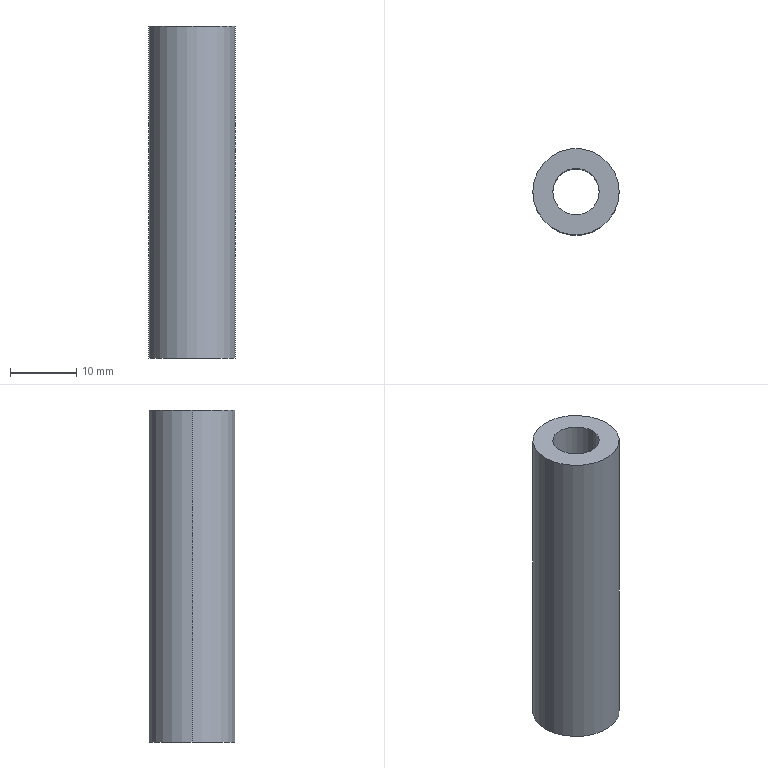Part | SolidWorks | features Extrusion 1 | 1 solid | 6 faces | box 13 x 13 x 50 mm | volume 4712 mm3 | cylinder 4 | plane 2 | commonest cylinder face diameters 7 x2 13 x2
STEP:
#1=CARTESIAN_POINT('',(-3.5,0.,50.));
#2=VERTEX_POINT('',#1);
#3=CARTESIAN_POINT('',(3.5,0.,50.));
#4=VERTEX_POINT('',#3);
#5=CARTESIAN_POINT('',(0.,0.,50.));
#6=DIRECTION('',(0.,0.,1.));
#7=DIRECTION('',(1.,0.,0.));
#8=AXIS2_PLACEMENT_3D('',#5,#6,#7);
#9=CIRCLE('',#8,3.5);
#10=EDGE_CURVE('',#2,#4,#9,.T.);
#11=ORIENTED_EDGE('',*,*,#10,.T.);
#12=CARTESIAN_POINT('',(3.5,0.,0.));
#13=VERTEX_POINT('',#12);
#14=CARTESIAN_POINT('',(3.5,0.,50.));
#15=DIRECTION('',(0.,0.,-1.));
#16=VECTOR('',#15,1000.);
#17=LINE('',#14,#16);
#18=EDGE_CURVE('',#4,#13,#17,.T.);
#19=ORIENTED_EDGE('',*,*,#18,.T.);
#20=CARTESIAN_POINT('',(-3.5,0.,0.));
#21=VERTEX_POINT('',#20);
#22=CARTESIAN_POINT('',(0.,0.,0.));
#23=DIRECTION('',(0.,0.,1.));
#24=DIRECTION('',(1.,0.,0.));
#25=AXIS2_PLACEMENT_3D('',#22,#23,#24);
#26=CIRCLE('',#25,3.5);
#27=EDGE_CURVE('',#21,#13,#26,.T.);
#28=ORIENTED_EDGE('',*,*,#27,.F.);
#29=CARTESIAN_POINT('',(-3.5,0.,50.));
#30=DIRECTION('',(0.,0.,-1.));
#31=VECTOR('',#30,1000.);
#32=LINE('',#29,#31);
#33=EDGE_CURVE('',#2,#21,#32,.T.);
#34=ORIENTED_EDGE('',*,*,#33,.F.);
#35=EDGE_LOOP('',(#11,#19,#28,#34));
#36=FACE_OUTER_BOUND('',#35,.T.);
#37=CARTESIAN_POINT('',(0.,0.,50.));
#38=DIRECTION('',(0.,0.,-1.));
#39=DIRECTION('',(-1.,0.,0.));
#40=AXIS2_PLACEMENT_3D('',#37,#38,#39);
#41=CYLINDRICAL_SURFACE('',#40,3.5);
#42=ADVANCED_FACE('',(#36),#41,.F.);
#43=CARTESIAN_POINT('',(6.5,0.,50.));
#44=VERTEX_POINT('',#43);
#45=CARTESIAN_POINT('',(-6.5,0.,50.));
#46=VERTEX_POINT('',#45);
#47=CARTESIAN_POINT('',(0.,0.,50.));
#48=DIRECTION('',(0.,0.,1.));
#49=DIRECTION('',(1.,0.,0.));
#50=AXIS2_PLACEMENT_3D('',#47,#48,#49);
#51=CIRCLE('',#50,6.5);
#52=EDGE_CURVE('',#44,#46,#51,.T.);
#53=ORIENTED_EDGE('',*,*,#52,.F.);
#54=CARTESIAN_POINT('',(6.5,0.,0.));
#55=VERTEX_POINT('',#54);
#56=CARTESIAN_POINT('',(6.5,0.,50.));
#57=DIRECTION('',(0.,0.,-1.));
#58=VECTOR('',#57,1000.);
#59=LINE('',#56,#58);
#60=EDGE_CURVE('',#44,#55,#59,.T.);
#61=ORIENTED_EDGE('',*,*,#60,.T.);
#62=CARTESIAN_POINT('',(-6.5,0.,0.));
#63=VERTEX_POINT('',#62);
#64=CARTESIAN_POINT('',(0.,0.,0.));
#65=DIRECTION('',(0.,0.,1.));
#66=DIRECTION('',(1.,0.,0.));
#67=AXIS2_PLACEMENT_3D('',#64,#65,#66);
#68=CIRCLE('',#67,6.5);
#69=EDGE_CURVE('',#55,#63,#68,.T.);
#70=ORIENTED_EDGE('',*,*,#69,.T.);
#71=CARTESIAN_POINT('',(-6.5,0.,50.));
#72=DIRECTION('',(0.,0.,-1.));
#73=VECTOR('',#72,1000.);
#74=LINE('',#71,#73);
#75=EDGE_CURVE('',#46,#63,#74,.T.);
#76=ORIENTED_EDGE('',*,*,#75,.F.);
#77=EDGE_LOOP('',(#53,#61,#70,#76));
#78=FACE_OUTER_BOUND('',#77,.T.);
#79=CARTESIAN_POINT('',(0.,0.,50.));
#80=DIRECTION('',(0.,0.,-1.));
#81=DIRECTION('',(-1.,0.,0.));
#82=AXIS2_PLACEMENT_3D('',#79,#80,#81);
#83=CYLINDRICAL_SURFACE('',#82,6.5);
#84=ADVANCED_FACE('',(#78),#83,.T.);
#85=CARTESIAN_POINT('',(0.,0.,50.));
#86=DIRECTION('',(0.,0.,1.));
#87=DIRECTION('',(1.,0.,0.));
#88=AXIS2_PLACEMENT_3D('',#85,#86,#87);
#89=CIRCLE('',#88,6.5);
#90=EDGE_CURVE('',#46,#44,#89,.T.);
#91=ORIENTED_EDGE('',*,*,#90,.T.);
#92=ORIENTED_EDGE('',*,*,#52,.T.);
#93=EDGE_LOOP('',(#91,#92));
#94=FACE_OUTER_BOUND('',#93,.T.);
#95=ORIENTED_EDGE('',*,*,#10,.F.);
#96=CARTESIAN_POINT('',(0.,0.,50.));
#97=DIRECTION('',(0.,0.,1.));
#98=DIRECTION('',(1.,0.,0.));
#99=AXIS2_PLACEMENT_3D('',#96,#97,#98);
#100=CIRCLE('',#99,3.5);
#101=EDGE_CURVE('',#4,#2,#100,.T.);
#102=ORIENTED_EDGE('',*,*,#101,.F.);
#103=EDGE_LOOP('',(#95,#102));
#104=FACE_BOUND('',#103,.T.);
#105=CARTESIAN_POINT('',(0.,0.,50.));
#106=DIRECTION('',(0.,0.,1.));
#107=DIRECTION('',(1.,0.,0.));
#108=AXIS2_PLACEMENT_3D('',#105,#106,#107);
#109=PLANE('',#108);
#110=ADVANCED_FACE('',(#94,#104),#109,.T.);
#111=CARTESIAN_POINT('',(0.,0.,0.));
#112=DIRECTION('',(0.,0.,1.));
#113=DIRECTION('',(1.,0.,0.));
#114=AXIS2_PLACEMENT_3D('',#111,#112,#113);
#115=CIRCLE('',#114,6.5);
#116=EDGE_CURVE('',#63,#55,#115,.T.);
#117=ORIENTED_EDGE('',*,*,#116,.F.);
#118=ORIENTED_EDGE('',*,*,#69,.F.);
#119=EDGE_LOOP('',(#117,#118));
#120=FACE_OUTER_BOUND('',#119,.T.);
#121=ORIENTED_EDGE('',*,*,#27,.T.);
#122=CARTESIAN_POINT('',(0.,0.,0.));
#123=DIRECTION('',(0.,0.,1.));
#124=DIRECTION('',(1.,0.,0.));
#125=AXIS2_PLACEMENT_3D('',#122,#123,#124);
#126=CIRCLE('',#125,3.5);
#127=EDGE_CURVE('',#13,#21,#126,.T.);
#128=ORIENTED_EDGE('',*,*,#127,.T.);
#129=EDGE_LOOP('',(#121,#128));
#130=FACE_BOUND('',#129,.T.);
#131=CARTESIAN_POINT('',(0.,0.,0.));
#132=DIRECTION('',(0.,0.,1.));
#133=DIRECTION('',(1.,0.,0.));
#134=AXIS2_PLACEMENT_3D('',#131,#132,#133);
#135=PLANE('',#134);
#136=ADVANCED_FACE('',(#120,#130),#135,.F.);
#137=ORIENTED_EDGE('',*,*,#60,.F.);
#138=ORIENTED_EDGE('',*,*,#90,.F.);
#139=ORIENTED_EDGE('',*,*,#75,.T.);
#140=ORIENTED_EDGE('',*,*,#116,.T.);
#141=EDGE_LOOP('',(#137,#138,#139,#140));
#142=FACE_OUTER_BOUND('',#141,.T.);
#143=CARTESIAN_POINT('',(0.,0.,50.));
#144=DIRECTION('',(0.,0.,-1.));
#145=DIRECTION('',(-1.,0.,0.));
#146=AXIS2_PLACEMENT_3D('',#143,#144,#145);
#147=CYLINDRICAL_SURFACE('',#146,6.5);
#148=ADVANCED_FACE('',(#142),#147,.T.);
#149=ORIENTED_EDGE('',*,*,#18,.F.);
#150=ORIENTED_EDGE('',*,*,#101,.T.);
#151=ORIENTED_EDGE('',*,*,#33,.T.);
#152=ORIENTED_EDGE('',*,*,#127,.F.);
#153=EDGE_LOOP('',(#149,#150,#151,#152));
#154=FACE_OUTER_BOUND('',#153,.T.);
#155=CARTESIAN_POINT('',(0.,0.,50.));
#156=DIRECTION('',(0.,0.,-1.));
#157=DIRECTION('',(-1.,0.,0.));
#158=AXIS2_PLACEMENT_3D('',#155,#156,#157);
#159=CYLINDRICAL_SURFACE('',#158,3.5);
#160=ADVANCED_FACE('',(#154),#159,.F.);
#161=CLOSED_SHELL('',(#42,#84,#110,#136,#148,#160));
#162=MANIFOLD_SOLID_BREP('',#161);
#163=CARTESIAN_POINT('',(0.,0.,0.));
#164=DIRECTION('',(0.,0.,1.));
#165=DIRECTION('',(1.,0.,0.));
#166=AXIS2_PLACEMENT_3D('',#163,#164,#165);
#167=(LENGTH_UNIT()NAMED_UNIT(*)SI_UNIT(.MILLI.,.METRE.));
#168=UNCERTAINTY_MEASURE_WITH_UNIT(LENGTH_MEASURE(0.00001),#167,'','');
#169=(NAMED_UNIT(*)PLANE_ANGLE_UNIT()SI_UNIT($,.RADIAN.));
#170=(NAMED_UNIT(*)SI_UNIT($,.STERADIAN.)SOLID_ANGLE_UNIT());
#171=(GEOMETRIC_REPRESENTATION_CONTEXT(3)GLOBAL_UNCERTAINTY_ASSIGNED_CONTEXT((#168))GLOBAL_UNIT_ASSIGNED_CONTEXT((#167,#169,#170))REPRESENTATION_CONTEXT('',''));
#172=ADVANCED_BREP_SHAPE_REPRESENTATION('',(#162,#166),#171);